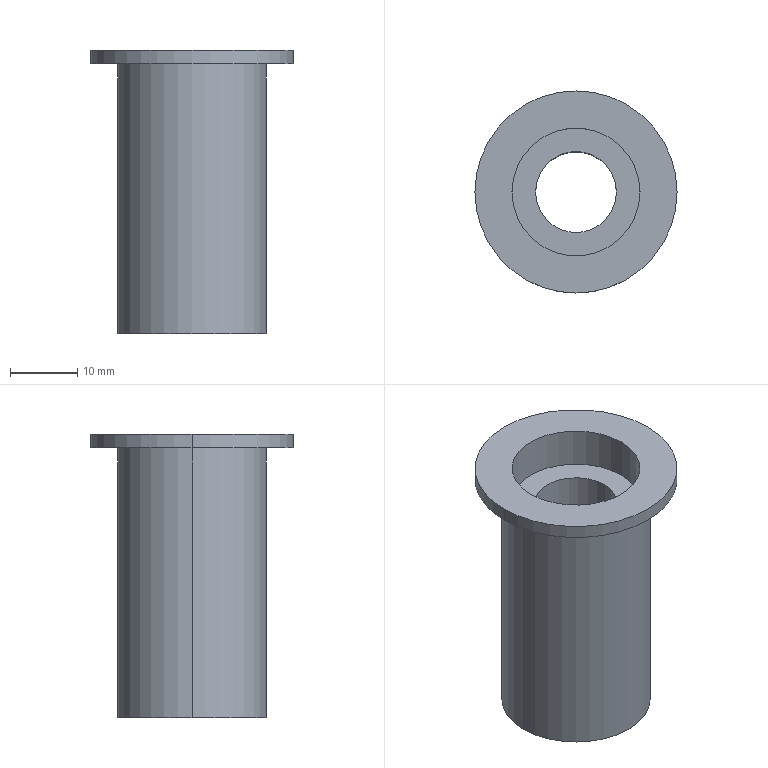Part | STEP file | Tube-changer locating roller SGN-2-21 | 1 solid | 15 faces | box 30 x 30 x 42 mm | volume 9824 mm3 | cylinder 10 | plane 5 | commonest cylinder face diameters 19 x4 12 x2 22 x2 30 x2
STEP:
#1=CARTESIAN_POINT('',(0.,0.,0.));
#2=DIRECTION('',(0.,0.,1.));
#3=DIRECTION('',(1.,0.,0.));
#4=AXIS2_PLACEMENT_3D('',#1,#2,#3);
#5=CARTESIAN_POINT('',(9.5,0.,36.));
#6=VERTEX_POINT('',#5);
#7=CARTESIAN_POINT('',(9.5,0.,42.));
#8=VERTEX_POINT('',#7);
#9=CARTESIAN_POINT('',(9.5,0.,36.));
#10=DIRECTION('',(0.,0.,1.));
#11=VECTOR('',#10,1.);
#12=LINE('',#9,#11);
#13=CARTESIAN_POINT('',(0.,0.,36.));
#14=DIRECTION('',(0.,0.,1.));
#15=DIRECTION('',(1.,0.,0.));
#16=AXIS2_PLACEMENT_3D('',#13,#14,#15);
#17=CYLINDRICAL_SURFACE('',#16,9.5);
#18=CARTESIAN_POINT('',(6.283,0.));
#19=DIRECTION('',(0.,1.));
#20=VECTOR('',#19,1.);
#21=LINE('',#18,#20);
#22=(GEOMETRIC_REPRESENTATION_CONTEXT(2)PARAMETRIC_REPRESENTATION_CONTEXT()REPRESENTATION_CONTEXT('',''));
#23=DEFINITIONAL_REPRESENTATION('',(#21),#22);
#24=PCURVE('',#17,#23);
#25=CARTESIAN_POINT('',(0.,0.,36.));
#26=DIRECTION('',(0.,0.,1.));
#27=DIRECTION('',(1.,0.,0.));
#28=AXIS2_PLACEMENT_3D('',#25,#26,#27);
#29=CYLINDRICAL_SURFACE('',#28,9.5);
#30=CARTESIAN_POINT('',(0.,0.));
#31=DIRECTION('',(0.,1.));
#32=VECTOR('',#31,1.);
#33=LINE('',#30,#32);
#34=(GEOMETRIC_REPRESENTATION_CONTEXT(2)PARAMETRIC_REPRESENTATION_CONTEXT()REPRESENTATION_CONTEXT('',''));
#35=DEFINITIONAL_REPRESENTATION('',(#33),#34);
#36=PCURVE('',#29,#35);
#37=SURFACE_CURVE('',#12,(#24,#36),.PCURVE_S1.);
#38=EDGE_CURVE('',#6,#8,#37,.T.);
#39=ORIENTED_EDGE('',*,*,#38,.T.);
#40=CARTESIAN_POINT('',(-9.5,0.,42.));
#41=VERTEX_POINT('',#40);
#42=CARTESIAN_POINT('',(0.,0.,42.));
#43=DIRECTION('',(0.,0.,1.));
#44=DIRECTION('',(1.,0.,0.));
#45=AXIS2_PLACEMENT_3D('',#42,#43,#44);
#46=CIRCLE('',#45,9.5);
#47=CARTESIAN_POINT('',(0.,6.));
#48=DIRECTION('',(1.,0.));
#49=VECTOR('',#48,1.);
#50=LINE('',#47,#49);
#51=(GEOMETRIC_REPRESENTATION_CONTEXT(2)PARAMETRIC_REPRESENTATION_CONTEXT()REPRESENTATION_CONTEXT('',''));
#52=DEFINITIONAL_REPRESENTATION('',(#50),#51);
#53=PCURVE('',#17,#52);
#54=CARTESIAN_POINT('',(0.,0.,42.));
#55=DIRECTION('',(0.,0.,1.));
#56=DIRECTION('',(1.,0.,0.));
#57=AXIS2_PLACEMENT_3D('',#54,#55,#56);
#58=PLANE('',#57);
#59=CARTESIAN_POINT('',(0.,0.));
#60=DIRECTION('',(1.,0.));
#61=AXIS2_PLACEMENT_2D('',#59,#60);
#62=CIRCLE('',#61,9.5);
#63=(GEOMETRIC_REPRESENTATION_CONTEXT(2)PARAMETRIC_REPRESENTATION_CONTEXT()REPRESENTATION_CONTEXT('',''));
#64=DEFINITIONAL_REPRESENTATION('',(#62),#63);
#65=PCURVE('',#58,#64);
#66=SURFACE_CURVE('',#46,(#53,#65),.PCURVE_S1.);
#67=EDGE_CURVE('',#41,#8,#66,.T.);
#68=ORIENTED_EDGE('',*,*,#67,.F.);
#69=CARTESIAN_POINT('',(-9.5,0.,36.));
#70=VERTEX_POINT('',#69);
#71=CARTESIAN_POINT('',(-9.5,0.,36.));
#72=DIRECTION('',(0.,0.,1.));
#73=VECTOR('',#72,1.);
#74=LINE('',#71,#73);
#75=CARTESIAN_POINT('',(3.142,0.));
#76=DIRECTION('',(0.,1.));
#77=VECTOR('',#76,1.);
#78=LINE('',#75,#77);
#79=(GEOMETRIC_REPRESENTATION_CONTEXT(2)PARAMETRIC_REPRESENTATION_CONTEXT()REPRESENTATION_CONTEXT('',''));
#80=DEFINITIONAL_REPRESENTATION('',(#78),#79);
#81=PCURVE('',#17,#80);
#82=CARTESIAN_POINT('',(3.142,0.));
#83=DIRECTION('',(0.,1.));
#84=VECTOR('',#83,1.);
#85=LINE('',#82,#84);
#86=(GEOMETRIC_REPRESENTATION_CONTEXT(2)PARAMETRIC_REPRESENTATION_CONTEXT()REPRESENTATION_CONTEXT('',''));
#87=DEFINITIONAL_REPRESENTATION('',(#85),#86);
#88=PCURVE('',#29,#87);
#89=SURFACE_CURVE('',#74,(#81,#88),.PCURVE_S1.);
#90=EDGE_CURVE('',#70,#41,#89,.T.);
#91=ORIENTED_EDGE('',*,*,#90,.F.);
#92=CARTESIAN_POINT('',(0.,0.,36.));
#93=DIRECTION('',(0.,0.,1.));
#94=DIRECTION('',(1.,0.,0.));
#95=AXIS2_PLACEMENT_3D('',#92,#93,#94);
#96=CIRCLE('',#95,9.5);
#97=CARTESIAN_POINT('',(0.,0.));
#98=DIRECTION('',(1.,0.));
#99=VECTOR('',#98,1.);
#100=LINE('',#97,#99);
#101=(GEOMETRIC_REPRESENTATION_CONTEXT(2)PARAMETRIC_REPRESENTATION_CONTEXT()REPRESENTATION_CONTEXT('',''));
#102=DEFINITIONAL_REPRESENTATION('',(#100),#101);
#103=PCURVE('',#17,#102);
#104=CARTESIAN_POINT('',(0.,0.,36.));
#105=DIRECTION('',(0.,0.,1.));
#106=DIRECTION('',(1.,0.,0.));
#107=AXIS2_PLACEMENT_3D('',#104,#105,#106);
#108=PLANE('',#107);
#109=CARTESIAN_POINT('',(0.,0.));
#110=DIRECTION('',(1.,0.));
#111=AXIS2_PLACEMENT_2D('',#109,#110);
#112=CIRCLE('',#111,9.5);
#113=(GEOMETRIC_REPRESENTATION_CONTEXT(2)PARAMETRIC_REPRESENTATION_CONTEXT()REPRESENTATION_CONTEXT('',''));
#114=DEFINITIONAL_REPRESENTATION('',(#112),#113);
#115=PCURVE('',#108,#114);
#116=SURFACE_CURVE('',#96,(#103,#115),.PCURVE_S1.);
#117=EDGE_CURVE('',#70,#6,#116,.T.);
#118=ORIENTED_EDGE('',*,*,#117,.T.);
#119=EDGE_LOOP('',(#39,#68,#91,#118));
#120=FACE_BOUND('',#119,.F.);
#121=ADVANCED_FACE('',(#120),#17,.F.);
#122=CARTESIAN_POINT('',(-9.5,0.,6.));
#123=VERTEX_POINT('',#122);
#124=CARTESIAN_POINT('',(-9.5,0.,0.));
#125=VERTEX_POINT('',#124);
#126=CARTESIAN_POINT('',(-9.5,0.,6.));
#127=DIRECTION('',(0.,0.,-1.));
#128=VECTOR('',#127,1.);
#129=LINE('',#126,#128);
#130=CARTESIAN_POINT('',(0.,0.,6.));
#131=DIRECTION('',(0.,0.,-1.));
#132=DIRECTION('',(-1.,0.,0.));
#133=AXIS2_PLACEMENT_3D('',#130,#131,#132);
#134=CYLINDRICAL_SURFACE('',#133,9.5);
#135=CARTESIAN_POINT('',(6.283,0.));
#136=DIRECTION('',(0.,1.));
#137=VECTOR('',#136,1.);
#138=LINE('',#135,#137);
#139=(GEOMETRIC_REPRESENTATION_CONTEXT(2)PARAMETRIC_REPRESENTATION_CONTEXT()REPRESENTATION_CONTEXT('',''));
#140=DEFINITIONAL_REPRESENTATION('',(#138),#139);
#141=PCURVE('',#134,#140);
#142=CARTESIAN_POINT('',(0.,0.,6.));
#143=DIRECTION('',(0.,0.,-1.));
#144=DIRECTION('',(-1.,0.,0.));
#145=AXIS2_PLACEMENT_3D('',#142,#143,#144);
#146=CYLINDRICAL_SURFACE('',#145,9.5);
#147=CARTESIAN_POINT('',(0.,0.));
#148=DIRECTION('',(0.,1.));
#149=VECTOR('',#148,1.);
#150=LINE('',#147,#149);
#151=(GEOMETRIC_REPRESENTATION_CONTEXT(2)PARAMETRIC_REPRESENTATION_CONTEXT()REPRESENTATION_CONTEXT('',''));
#152=DEFINITIONAL_REPRESENTATION('',(#150),#151);
#153=PCURVE('',#146,#152);
#154=SURFACE_CURVE('',#129,(#141,#153),.PCURVE_S1.);
#155=EDGE_CURVE('',#123,#125,#154,.T.);
#156=ORIENTED_EDGE('',*,*,#155,.T.);
#157=CARTESIAN_POINT('',(9.5,0.,0.));
#158=VERTEX_POINT('',#157);
#159=CARTESIAN_POINT('',(0.,0.,0.));
#160=DIRECTION('',(0.,0.,-1.));
#161=DIRECTION('',(-1.,0.,0.));
#162=AXIS2_PLACEMENT_3D('',#159,#160,#161);
#163=CIRCLE('',#162,9.5);
#164=CARTESIAN_POINT('',(0.,6.));
#165=DIRECTION('',(1.,0.));
#166=VECTOR('',#165,1.);
#167=LINE('',#164,#166);
#168=(GEOMETRIC_REPRESENTATION_CONTEXT(2)PARAMETRIC_REPRESENTATION_CONTEXT()REPRESENTATION_CONTEXT('',''));
#169=DEFINITIONAL_REPRESENTATION('',(#167),#168);
#170=PCURVE('',#134,#169);
#171=CARTESIAN_POINT('',(0.,0.,0.));
#172=DIRECTION('',(0.,0.,1.));
#173=DIRECTION('',(1.,0.,0.));
#174=AXIS2_PLACEMENT_3D('',#171,#172,#173);
#175=PLANE('',#174);
#176=CARTESIAN_POINT('',(-9.5,0.));
#177=CARTESIAN_POINT('',(-9.5,16.454));
#178=CARTESIAN_POINT('',(4.75,8.227));
#179=CARTESIAN_POINT('',(19.,0.));
#180=CARTESIAN_POINT('',(4.75,-8.227));
#181=CARTESIAN_POINT('',(-9.5,-16.454));
#182=CARTESIAN_POINT('',(-9.5,0.));
#183=(BOUNDED_CURVE()B_SPLINE_CURVE(2,(#176,#177,#178,#179,#180,#181,#182),.UNSPECIFIED.,.T.,.F.)B_SPLINE_CURVE_WITH_KNOTS((1,2,2,2,2,1),(-2.094,0.,2.094,4.189,6.283,8.378),.UNSPECIFIED.)CURVE()GEOMETRIC_REPRESENTATION_ITEM()RATIONAL_B_SPLINE_CURVE((1.,0.5,1.,0.5,1.,0.5,1.))REPRESENTATION_ITEM(''));
#184=(GEOMETRIC_REPRESENTATION_CONTEXT(2)PARAMETRIC_REPRESENTATION_CONTEXT()REPRESENTATION_CONTEXT('',''));
#185=DEFINITIONAL_REPRESENTATION('',(#183),#184);
#186=PCURVE('',#175,#185);
#187=SURFACE_CURVE('',#163,(#170,#186),.PCURVE_S1.);
#188=EDGE_CURVE('',#158,#125,#187,.T.);
#189=ORIENTED_EDGE('',*,*,#188,.F.);
#190=CARTESIAN_POINT('',(9.5,0.,6.));
#191=VERTEX_POINT('',#190);
#192=CARTESIAN_POINT('',(9.5,0.,6.));
#193=DIRECTION('',(0.,0.,-1.));
#194=VECTOR('',#193,1.);
#195=LINE('',#192,#194);
#196=CARTESIAN_POINT('',(3.142,0.));
#197=DIRECTION('',(0.,1.));
#198=VECTOR('',#197,1.);
#199=LINE('',#196,#198);
#200=(GEOMETRIC_REPRESENTATION_CONTEXT(2)PARAMETRIC_REPRESENTATION_CONTEXT()REPRESENTATION_CONTEXT('',''));
#201=DEFINITIONAL_REPRESENTATION('',(#199),#200);
#202=PCURVE('',#134,#201);
#203=CARTESIAN_POINT('',(3.142,0.));
#204=DIRECTION('',(0.,1.));
#205=VECTOR('',#204,1.);
#206=LINE('',#203,#205);
#207=(GEOMETRIC_REPRESENTATION_CONTEXT(2)PARAMETRIC_REPRESENTATION_CONTEXT()REPRESENTATION_CONTEXT('',''));
#208=DEFINITIONAL_REPRESENTATION('',(#206),#207);
#209=PCURVE('',#146,#208);
#210=SURFACE_CURVE('',#195,(#202,#209),.PCURVE_S1.);
#211=EDGE_CURVE('',#191,#158,#210,.T.);
#212=ORIENTED_EDGE('',*,*,#211,.F.);
#213=CARTESIAN_POINT('',(0.,0.,6.));
#214=DIRECTION('',(0.,0.,-1.));
#215=DIRECTION('',(-1.,0.,0.));
#216=AXIS2_PLACEMENT_3D('',#213,#214,#215);
#217=CIRCLE('',#216,9.5);
#218=CARTESIAN_POINT('',(0.,0.));
#219=DIRECTION('',(1.,0.));
#220=VECTOR('',#219,1.);
#221=LINE('',#218,#220);
#222=(GEOMETRIC_REPRESENTATION_CONTEXT(2)PARAMETRIC_REPRESENTATION_CONTEXT()REPRESENTATION_CONTEXT('',''));
#223=DEFINITIONAL_REPRESENTATION('',(#221),#222);
#224=PCURVE('',#134,#223);
#225=CARTESIAN_POINT('',(0.,0.,6.));
#226=DIRECTION('',(0.,0.,-1.));
#227=DIRECTION('',(-1.,0.,0.));
#228=AXIS2_PLACEMENT_3D('',#225,#226,#227);
#229=PLANE('',#228);
#230=CARTESIAN_POINT('',(0.,0.));
#231=DIRECTION('',(1.,0.));
#232=AXIS2_PLACEMENT_2D('',#230,#231);
#233=CIRCLE('',#232,9.5);
#234=(GEOMETRIC_REPRESENTATION_CONTEXT(2)PARAMETRIC_REPRESENTATION_CONTEXT()REPRESENTATION_CONTEXT('',''));
#235=DEFINITIONAL_REPRESENTATION('',(#233),#234);
#236=PCURVE('',#229,#235);
#237=SURFACE_CURVE('',#217,(#224,#236),.PCURVE_S1.);
#238=EDGE_CURVE('',#191,#123,#237,.T.);
#239=ORIENTED_EDGE('',*,*,#238,.T.);
#240=EDGE_LOOP('',(#156,#189,#212,#239));
#241=FACE_BOUND('',#240,.F.);
#242=ADVANCED_FACE('',(#241),#134,.F.);
#243=CARTESIAN_POINT('',(15.,0.,42.));
#244=VERTEX_POINT('',#243);
#245=CARTESIAN_POINT('',(-15.,0.,42.));
#246=VERTEX_POINT('',#245);
#247=CARTESIAN_POINT('',(0.,0.,42.));
#248=DIRECTION('',(0.,0.,1.));
#249=DIRECTION('',(1.,0.,0.));
#250=AXIS2_PLACEMENT_3D('',#247,#248,#249);
#251=CIRCLE('',#250,15.);
#252=CARTESIAN_POINT('',(0.,0.,42.));
#253=DIRECTION('',(0.,0.,-1.));
#254=DIRECTION('',(-1.,0.,0.));
#255=AXIS2_PLACEMENT_3D('',#252,#253,#254);
#256=CYLINDRICAL_SURFACE('',#255,15.);
#257=CARTESIAN_POINT('',(3.142,0.));
#258=DIRECTION('',(-1.,0.));
#259=VECTOR('',#258,1.);
#260=LINE('',#257,#259);
#261=(GEOMETRIC_REPRESENTATION_CONTEXT(2)PARAMETRIC_REPRESENTATION_CONTEXT()REPRESENTATION_CONTEXT('',''));
#262=DEFINITIONAL_REPRESENTATION('',(#260),#261);
#263=PCURVE('',#256,#262);
#264=CARTESIAN_POINT('',(0.,0.));
#265=DIRECTION('',(1.,0.));
#266=AXIS2_PLACEMENT_2D('',#264,#265);
#267=CIRCLE('',#266,15.);
#268=(GEOMETRIC_REPRESENTATION_CONTEXT(2)PARAMETRIC_REPRESENTATION_CONTEXT()REPRESENTATION_CONTEXT('',''));
#269=DEFINITIONAL_REPRESENTATION('',(#267),#268);
#270=PCURVE('',#58,#269);
#271=SURFACE_CURVE('',#251,(#263,#270),.PCURVE_S1.);
#272=EDGE_CURVE('',#244,#246,#271,.T.);
#273=ORIENTED_EDGE('',*,*,#272,.F.);
#274=CARTESIAN_POINT('',(15.,0.,40.));
#275=VERTEX_POINT('',#274);
#276=CARTESIAN_POINT('',(15.,0.,42.));
#277=DIRECTION('',(0.,0.,-1.));
#278=VECTOR('',#277,1.);
#279=LINE('',#276,#278);
#280=CARTESIAN_POINT('',(3.142,0.));
#281=DIRECTION('',(0.,1.));
#282=VECTOR('',#281,1.);
#283=LINE('',#280,#282);
#284=(GEOMETRIC_REPRESENTATION_CONTEXT(2)PARAMETRIC_REPRESENTATION_CONTEXT()REPRESENTATION_CONTEXT('',''));
#285=DEFINITIONAL_REPRESENTATION('',(#283),#284);
#286=PCURVE('',#256,#285);
#287=CARTESIAN_POINT('',(0.,0.,42.));
#288=DIRECTION('',(0.,0.,-1.));
#289=DIRECTION('',(-1.,0.,0.));
#290=AXIS2_PLACEMENT_3D('',#287,#288,#289);
#291=CYLINDRICAL_SURFACE('',#290,15.);
#292=CARTESIAN_POINT('',(3.142,0.));
#293=DIRECTION('',(0.,1.));
#294=VECTOR('',#293,1.);
#295=LINE('',#292,#294);
#296=(GEOMETRIC_REPRESENTATION_CONTEXT(2)PARAMETRIC_REPRESENTATION_CONTEXT()REPRESENTATION_CONTEXT('',''));
#297=DEFINITIONAL_REPRESENTATION('',(#295),#296);
#298=PCURVE('',#291,#297);
#299=SURFACE_CURVE('',#279,(#286,#298),.PCURVE_S1.);
#300=EDGE_CURVE('',#244,#275,#299,.T.);
#301=ORIENTED_EDGE('',*,*,#300,.T.);
#302=CARTESIAN_POINT('',(-15.,0.,40.));
#303=VERTEX_POINT('',#302);
#304=CARTESIAN_POINT('',(0.,0.,40.));
#305=DIRECTION('',(0.,0.,1.));
#306=DIRECTION('',(1.,0.,0.));
#307=AXIS2_PLACEMENT_3D('',#304,#305,#306);
#308=CIRCLE('',#307,15.);
#309=CARTESIAN_POINT('',(3.142,2.));
#310=DIRECTION('',(-1.,0.));
#311=VECTOR('',#310,1.);
#312=LINE('',#309,#311);
#313=(GEOMETRIC_REPRESENTATION_CONTEXT(2)PARAMETRIC_REPRESENTATION_CONTEXT()REPRESENTATION_CONTEXT('',''));
#314=DEFINITIONAL_REPRESENTATION('',(#312),#313);
#315=PCURVE('',#256,#314);
#316=CARTESIAN_POINT('',(0.,0.,40.));
#317=DIRECTION('',(0.,0.,1.));
#318=DIRECTION('',(1.,0.,0.));
#319=AXIS2_PLACEMENT_3D('',#316,#317,#318);
#320=PLANE('',#319);
#321=CARTESIAN_POINT('',(0.,0.));
#322=DIRECTION('',(1.,0.));
#323=AXIS2_PLACEMENT_2D('',#321,#322);
#324=CIRCLE('',#323,15.);
#325=(GEOMETRIC_REPRESENTATION_CONTEXT(2)PARAMETRIC_REPRESENTATION_CONTEXT()REPRESENTATION_CONTEXT('',''));
#326=DEFINITIONAL_REPRESENTATION('',(#324),#325);
#327=PCURVE('',#320,#326);
#328=SURFACE_CURVE('',#308,(#315,#327),.PCURVE_S1.);
#329=EDGE_CURVE('',#275,#303,#328,.T.);
#330=ORIENTED_EDGE('',*,*,#329,.T.);
#331=CARTESIAN_POINT('',(-15.,0.,42.));
#332=DIRECTION('',(0.,0.,-1.));
#333=VECTOR('',#332,1.);
#334=LINE('',#331,#333);
#335=CARTESIAN_POINT('',(0.,0.));
#336=DIRECTION('',(0.,1.));
#337=VECTOR('',#336,1.);
#338=LINE('',#335,#337);
#339=(GEOMETRIC_REPRESENTATION_CONTEXT(2)PARAMETRIC_REPRESENTATION_CONTEXT()REPRESENTATION_CONTEXT('',''));
#340=DEFINITIONAL_REPRESENTATION('',(#338),#339);
#341=PCURVE('',#256,#340);
#342=CARTESIAN_POINT('',(6.283,0.));
#343=DIRECTION('',(0.,1.));
#344=VECTOR('',#343,1.);
#345=LINE('',#342,#344);
#346=(GEOMETRIC_REPRESENTATION_CONTEXT(2)PARAMETRIC_REPRESENTATION_CONTEXT()REPRESENTATION_CONTEXT('',''));
#347=DEFINITIONAL_REPRESENTATION('',(#345),#346);
#348=PCURVE('',#291,#347);
#349=SURFACE_CURVE('',#334,(#341,#348),.PCURVE_S1.);
#350=EDGE_CURVE('',#246,#303,#349,.T.);
#351=ORIENTED_EDGE('',*,*,#350,.F.);
#352=EDGE_LOOP('',(#273,#301,#330,#351));
#353=FACE_BOUND('',#352,.T.);
#354=ADVANCED_FACE('',(#353),#256,.T.);
#355=CARTESIAN_POINT('',(11.,0.,40.));
#356=VERTEX_POINT('',#355);
#357=CARTESIAN_POINT('',(-11.,0.,40.));
#358=VERTEX_POINT('',#357);
#359=CARTESIAN_POINT('',(0.,0.,40.));
#360=DIRECTION('',(0.,0.,1.));
#361=DIRECTION('',(1.,0.,0.));
#362=AXIS2_PLACEMENT_3D('',#359,#360,#361);
#363=CIRCLE('',#362,11.);
#364=CARTESIAN_POINT('',(0.,0.,40.));
#365=DIRECTION('',(0.,0.,-1.));
#366=DIRECTION('',(-1.,0.,0.));
#367=AXIS2_PLACEMENT_3D('',#364,#365,#366);
#368=CYLINDRICAL_SURFACE('',#367,11.);
#369=CARTESIAN_POINT('',(3.142,0.));
#370=DIRECTION('',(-1.,0.));
#371=VECTOR('',#370,1.);
#372=LINE('',#369,#371);
#373=(GEOMETRIC_REPRESENTATION_CONTEXT(2)PARAMETRIC_REPRESENTATION_CONTEXT()REPRESENTATION_CONTEXT('',''));
#374=DEFINITIONAL_REPRESENTATION('',(#372),#373);
#375=PCURVE('',#368,#374);
#376=CARTESIAN_POINT('',(0.,0.));
#377=DIRECTION('',(1.,0.));
#378=AXIS2_PLACEMENT_2D('',#376,#377);
#379=CIRCLE('',#378,11.);
#380=(GEOMETRIC_REPRESENTATION_CONTEXT(2)PARAMETRIC_REPRESENTATION_CONTEXT()REPRESENTATION_CONTEXT('',''));
#381=DEFINITIONAL_REPRESENTATION('',(#379),#380);
#382=PCURVE('',#320,#381);
#383=SURFACE_CURVE('',#363,(#375,#382),.PCURVE_S1.);
#384=EDGE_CURVE('',#356,#358,#383,.T.);
#385=ORIENTED_EDGE('',*,*,#384,.F.);
#386=CARTESIAN_POINT('',(11.,0.,0.));
#387=VERTEX_POINT('',#386);
#388=CARTESIAN_POINT('',(11.,0.,40.));
#389=DIRECTION('',(0.,0.,-1.));
#390=VECTOR('',#389,1.);
#391=LINE('',#388,#390);
#392=CARTESIAN_POINT('',(3.142,0.));
#393=DIRECTION('',(0.,1.));
#394=VECTOR('',#393,1.);
#395=LINE('',#392,#394);
#396=(GEOMETRIC_REPRESENTATION_CONTEXT(2)PARAMETRIC_REPRESENTATION_CONTEXT()REPRESENTATION_CONTEXT('',''));
#397=DEFINITIONAL_REPRESENTATION('',(#395),#396);
#398=PCURVE('',#368,#397);
#399=CARTESIAN_POINT('',(0.,0.,40.));
#400=DIRECTION('',(0.,0.,-1.));
#401=DIRECTION('',(-1.,0.,0.));
#402=AXIS2_PLACEMENT_3D('',#399,#400,#401);
#403=CYLINDRICAL_SURFACE('',#402,11.);
#404=CARTESIAN_POINT('',(3.142,0.));
#405=DIRECTION('',(0.,1.));
#406=VECTOR('',#405,1.);
#407=LINE('',#404,#406);
#408=(GEOMETRIC_REPRESENTATION_CONTEXT(2)PARAMETRIC_REPRESENTATION_CONTEXT()REPRESENTATION_CONTEXT('',''));
#409=DEFINITIONAL_REPRESENTATION('',(#407),#408);
#410=PCURVE('',#403,#409);
#411=SURFACE_CURVE('',#391,(#398,#410),.PCURVE_S1.);
#412=EDGE_CURVE('',#356,#387,#411,.T.);
#413=ORIENTED_EDGE('',*,*,#412,.T.);
#414=CARTESIAN_POINT('',(-11.,0.,0.));
#415=VERTEX_POINT('',#414);
#416=CARTESIAN_POINT('',(0.,0.,0.));
#417=DIRECTION('',(0.,0.,1.));
#418=DIRECTION('',(1.,0.,0.));
#419=AXIS2_PLACEMENT_3D('',#416,#417,#418);
#420=CIRCLE('',#419,11.);
#421=CARTESIAN_POINT('',(3.142,40.));
#422=DIRECTION('',(-1.,0.));
#423=VECTOR('',#422,1.);
#424=LINE('',#421,#423);
#425=(GEOMETRIC_REPRESENTATION_CONTEXT(2)PARAMETRIC_REPRESENTATION_CONTEXT()REPRESENTATION_CONTEXT('',''));
#426=DEFINITIONAL_REPRESENTATION('',(#424),#425);
#427=PCURVE('',#368,#426);
#428=CARTESIAN_POINT('',(0.,0.));
#429=DIRECTION('',(1.,0.));
#430=AXIS2_PLACEMENT_2D('',#428,#429);
#431=CIRCLE('',#430,11.);
#432=(GEOMETRIC_REPRESENTATION_CONTEXT(2)PARAMETRIC_REPRESENTATION_CONTEXT()REPRESENTATION_CONTEXT('',''));
#433=DEFINITIONAL_REPRESENTATION('',(#431),#432);
#434=PCURVE('',#175,#433);
#435=SURFACE_CURVE('',#420,(#427,#434),.PCURVE_S1.);
#436=EDGE_CURVE('',#387,#415,#435,.T.);
#437=ORIENTED_EDGE('',*,*,#436,.T.);
#438=CARTESIAN_POINT('',(-11.,0.,40.));
#439=DIRECTION('',(0.,0.,-1.));
#440=VECTOR('',#439,1.);
#441=LINE('',#438,#440);
#442=CARTESIAN_POINT('',(0.,0.));
#443=DIRECTION('',(0.,1.));
#444=VECTOR('',#443,1.);
#445=LINE('',#442,#444);
#446=(GEOMETRIC_REPRESENTATION_CONTEXT(2)PARAMETRIC_REPRESENTATION_CONTEXT()REPRESENTATION_CONTEXT('',''));
#447=DEFINITIONAL_REPRESENTATION('',(#445),#446);
#448=PCURVE('',#368,#447);
#449=CARTESIAN_POINT('',(6.283,0.));
#450=DIRECTION('',(0.,1.));
#451=VECTOR('',#450,1.);
#452=LINE('',#449,#451);
#453=(GEOMETRIC_REPRESENTATION_CONTEXT(2)PARAMETRIC_REPRESENTATION_CONTEXT()REPRESENTATION_CONTEXT('',''));
#454=DEFINITIONAL_REPRESENTATION('',(#452),#453);
#455=PCURVE('',#403,#454);
#456=SURFACE_CURVE('',#441,(#448,#455),.PCURVE_S1.);
#457=EDGE_CURVE('',#358,#415,#456,.T.);
#458=ORIENTED_EDGE('',*,*,#457,.F.);
#459=EDGE_LOOP('',(#385,#413,#437,#458));
#460=FACE_BOUND('',#459,.T.);
#461=ADVANCED_FACE('',(#460),#368,.T.);
#462=CARTESIAN_POINT('',(-6.,0.,36.));
#463=VERTEX_POINT('',#462);
#464=CARTESIAN_POINT('',(-6.,0.,6.));
#465=VERTEX_POINT('',#464);
#466=CARTESIAN_POINT('',(-6.,0.,40.));
#467=DIRECTION('',(0.,0.,-1.));
#468=VECTOR('',#467,1.);
#469=LINE('',#466,#468);
#470=CARTESIAN_POINT('',(0.,0.,40.));
#471=DIRECTION('',(0.,0.,-1.));
#472=DIRECTION('',(-1.,0.,0.));
#473=AXIS2_PLACEMENT_3D('',#470,#471,#472);
#474=CYLINDRICAL_SURFACE('',#473,6.);
#475=CARTESIAN_POINT('',(6.283,0.));
#476=DIRECTION('',(0.,1.));
#477=VECTOR('',#476,1.);
#478=LINE('',#475,#477);
#479=(GEOMETRIC_REPRESENTATION_CONTEXT(2)PARAMETRIC_REPRESENTATION_CONTEXT()REPRESENTATION_CONTEXT('',''));
#480=DEFINITIONAL_REPRESENTATION('',(#478),#479);
#481=PCURVE('',#474,#480);
#482=CARTESIAN_POINT('',(0.,0.,40.));
#483=DIRECTION('',(0.,0.,-1.));
#484=DIRECTION('',(-1.,0.,0.));
#485=AXIS2_PLACEMENT_3D('',#482,#483,#484);
#486=CYLINDRICAL_SURFACE('',#485,6.);
#487=CARTESIAN_POINT('',(0.,0.));
#488=DIRECTION('',(0.,1.));
#489=VECTOR('',#488,1.);
#490=LINE('',#487,#489);
#491=(GEOMETRIC_REPRESENTATION_CONTEXT(2)PARAMETRIC_REPRESENTATION_CONTEXT()REPRESENTATION_CONTEXT('',''));
#492=DEFINITIONAL_REPRESENTATION('',(#490),#491);
#493=PCURVE('',#486,#492);
#494=SURFACE_CURVE('',#469,(#481,#493),.PCURVE_S1.);
#495=EDGE_CURVE('',#463,#465,#494,.T.);
#496=ORIENTED_EDGE('',*,*,#495,.T.);
#497=CARTESIAN_POINT('',(6.,0.,6.));
#498=VERTEX_POINT('',#497);
#499=CARTESIAN_POINT('',(0.,0.,6.));
#500=DIRECTION('',(0.,0.,-1.));
#501=DIRECTION('',(-1.,0.,0.));
#502=AXIS2_PLACEMENT_3D('',#499,#500,#501);
#503=CIRCLE('',#502,6.);
#504=CARTESIAN_POINT('',(0.,34.));
#505=DIRECTION('',(1.,0.));
#506=VECTOR('',#505,1.);
#507=LINE('',#504,#506);
#508=(GEOMETRIC_REPRESENTATION_CONTEXT(2)PARAMETRIC_REPRESENTATION_CONTEXT()REPRESENTATION_CONTEXT('',''));
#509=DEFINITIONAL_REPRESENTATION('',(#507),#508);
#510=PCURVE('',#474,#509);
#511=CARTESIAN_POINT('',(0.,0.));
#512=DIRECTION('',(1.,0.));
#513=AXIS2_PLACEMENT_2D('',#511,#512);
#514=CIRCLE('',#513,6.);
#515=(GEOMETRIC_REPRESENTATION_CONTEXT(2)PARAMETRIC_REPRESENTATION_CONTEXT()REPRESENTATION_CONTEXT('',''));
#516=DEFINITIONAL_REPRESENTATION('',(#514),#515);
#517=PCURVE('',#229,#516);
#518=SURFACE_CURVE('',#503,(#510,#517),.PCURVE_S1.);
#519=EDGE_CURVE('',#498,#465,#518,.T.);
#520=ORIENTED_EDGE('',*,*,#519,.F.);
#521=CARTESIAN_POINT('',(6.,0.,36.));
#522=VERTEX_POINT('',#521);
#523=CARTESIAN_POINT('',(6.,0.,40.));
#524=DIRECTION('',(0.,0.,-1.));
#525=VECTOR('',#524,1.);
#526=LINE('',#523,#525);
#527=CARTESIAN_POINT('',(3.142,0.));
#528=DIRECTION('',(0.,1.));
#529=VECTOR('',#528,1.);
#530=LINE('',#527,#529);
#531=(GEOMETRIC_REPRESENTATION_CONTEXT(2)PARAMETRIC_REPRESENTATION_CONTEXT()REPRESENTATION_CONTEXT('',''));
#532=DEFINITIONAL_REPRESENTATION('',(#530),#531);
#533=PCURVE('',#474,#532);
#534=CARTESIAN_POINT('',(3.142,0.));
#535=DIRECTION('',(0.,1.));
#536=VECTOR('',#535,1.);
#537=LINE('',#534,#536);
#538=(GEOMETRIC_REPRESENTATION_CONTEXT(2)PARAMETRIC_REPRESENTATION_CONTEXT()REPRESENTATION_CONTEXT('',''));
#539=DEFINITIONAL_REPRESENTATION('',(#537),#538);
#540=PCURVE('',#486,#539);
#541=SURFACE_CURVE('',#526,(#533,#540),.PCURVE_S1.);
#542=EDGE_CURVE('',#522,#498,#541,.T.);
#543=ORIENTED_EDGE('',*,*,#542,.F.);
#544=CARTESIAN_POINT('',(0.,0.,36.));
#545=DIRECTION('',(0.,0.,1.));
#546=DIRECTION('',(1.,0.,0.));
#547=AXIS2_PLACEMENT_3D('',#544,#545,#546);
#548=CIRCLE('',#547,6.);
#549=CARTESIAN_POINT('',(9.425,4.));
#550=DIRECTION('',(-1.,0.));
#551=VECTOR('',#550,1.);
#552=LINE('',#549,#551);
#553=(GEOMETRIC_REPRESENTATION_CONTEXT(2)PARAMETRIC_REPRESENTATION_CONTEXT()REPRESENTATION_CONTEXT('',''));
#554=DEFINITIONAL_REPRESENTATION('',(#552),#553);
#555=PCURVE('',#474,#554);
#556=CARTESIAN_POINT('',(0.,0.));
#557=DIRECTION('',(1.,0.));
#558=AXIS2_PLACEMENT_2D('',#556,#557);
#559=CIRCLE('',#558,6.);
#560=(GEOMETRIC_REPRESENTATION_CONTEXT(2)PARAMETRIC_REPRESENTATION_CONTEXT()REPRESENTATION_CONTEXT('',''));
#561=DEFINITIONAL_REPRESENTATION('',(#559),#560);
#562=PCURVE('',#108,#561);
#563=SURFACE_CURVE('',#548,(#555,#562),.PCURVE_S1.);
#564=EDGE_CURVE('',#463,#522,#563,.T.);
#565=ORIENTED_EDGE('',*,*,#564,.F.);
#566=EDGE_LOOP('',(#496,#520,#543,#565));
#567=FACE_BOUND('',#566,.F.);
#568=ADVANCED_FACE('',(#567),#474,.F.);
#569=CARTESIAN_POINT('',(0.,0.,6.));
#570=DIRECTION('',(0.,0.,-1.));
#571=DIRECTION('',(-1.,0.,0.));
#572=AXIS2_PLACEMENT_3D('',#569,#570,#571);
#573=CIRCLE('',#572,6.);
#574=CARTESIAN_POINT('',(0.,34.));
#575=DIRECTION('',(1.,0.));
#576=VECTOR('',#575,1.);
#577=LINE('',#574,#576);
#578=(GEOMETRIC_REPRESENTATION_CONTEXT(2)PARAMETRIC_REPRESENTATION_CONTEXT()REPRESENTATION_CONTEXT('',''));
#579=DEFINITIONAL_REPRESENTATION('',(#577),#578);
#580=PCURVE('',#486,#579);
#581=CARTESIAN_POINT('',(0.,0.));
#582=DIRECTION('',(1.,0.));
#583=AXIS2_PLACEMENT_2D('',#581,#582);
#584=CIRCLE('',#583,6.);
#585=(GEOMETRIC_REPRESENTATION_CONTEXT(2)PARAMETRIC_REPRESENTATION_CONTEXT()REPRESENTATION_CONTEXT('',''));
#586=DEFINITIONAL_REPRESENTATION('',(#584),#585);
#587=PCURVE('',#229,#586);
#588=SURFACE_CURVE('',#573,(#580,#587),.PCURVE_S1.);
#589=EDGE_CURVE('',#465,#498,#588,.T.);
#590=ORIENTED_EDGE('',*,*,#589,.F.);
#591=ORIENTED_EDGE('',*,*,#495,.F.);
#592=CARTESIAN_POINT('',(0.,0.,36.));
#593=DIRECTION('',(0.,0.,1.));
#594=DIRECTION('',(1.,0.,0.));
#595=AXIS2_PLACEMENT_3D('',#592,#593,#594);
#596=CIRCLE('',#595,6.);
#597=CARTESIAN_POINT('',(3.142,4.));
#598=DIRECTION('',(-1.,0.));
#599=VECTOR('',#598,1.);
#600=LINE('',#597,#599);
#601=(GEOMETRIC_REPRESENTATION_CONTEXT(2)PARAMETRIC_REPRESENTATION_CONTEXT()REPRESENTATION_CONTEXT('',''));
#602=DEFINITIONAL_REPRESENTATION('',(#600),#601);
#603=PCURVE('',#486,#602);
#604=CARTESIAN_POINT('',(0.,0.));
#605=DIRECTION('',(1.,0.));
#606=AXIS2_PLACEMENT_2D('',#604,#605);
#607=CIRCLE('',#606,6.);
#608=(GEOMETRIC_REPRESENTATION_CONTEXT(2)PARAMETRIC_REPRESENTATION_CONTEXT()REPRESENTATION_CONTEXT('',''));
#609=DEFINITIONAL_REPRESENTATION('',(#607),#608);
#610=PCURVE('',#108,#609);
#611=SURFACE_CURVE('',#596,(#603,#610),.PCURVE_S1.);
#612=EDGE_CURVE('',#522,#463,#611,.T.);
#613=ORIENTED_EDGE('',*,*,#612,.F.);
#614=ORIENTED_EDGE('',*,*,#542,.T.);
#615=EDGE_LOOP('',(#590,#591,#613,#614));
#616=FACE_BOUND('',#615,.F.);
#617=ADVANCED_FACE('',(#616),#486,.F.);
#618=CARTESIAN_POINT('',(0.,0.,0.));
#619=DIRECTION('',(0.,0.,-1.));
#620=DIRECTION('',(-1.,0.,0.));
#621=AXIS2_PLACEMENT_3D('',#618,#619,#620);
#622=CIRCLE('',#621,9.5);
#623=CARTESIAN_POINT('',(-9.5,0.));
#624=CARTESIAN_POINT('',(-9.5,16.454));
#625=CARTESIAN_POINT('',(4.75,8.227));
#626=CARTESIAN_POINT('',(19.,0.));
#627=CARTESIAN_POINT('',(4.75,-8.227));
#628=CARTESIAN_POINT('',(-9.5,-16.454));
#629=CARTESIAN_POINT('',(-9.5,0.));
#630=(BOUNDED_CURVE()B_SPLINE_CURVE(2,(#623,#624,#625,#626,#627,#628,#629),.UNSPECIFIED.,.T.,.F.)B_SPLINE_CURVE_WITH_KNOTS((1,2,2,2,2,1),(-2.094,0.,2.094,4.189,6.283,8.378),.UNSPECIFIED.)CURVE()GEOMETRIC_REPRESENTATION_ITEM()RATIONAL_B_SPLINE_CURVE((1.,0.5,1.,0.5,1.,0.5,1.))REPRESENTATION_ITEM(''));
#631=(GEOMETRIC_REPRESENTATION_CONTEXT(2)PARAMETRIC_REPRESENTATION_CONTEXT()REPRESENTATION_CONTEXT('',''));
#632=DEFINITIONAL_REPRESENTATION('',(#630),#631);
#633=PCURVE('',#175,#632);
#634=CARTESIAN_POINT('',(0.,6.));
#635=DIRECTION('',(1.,0.));
#636=VECTOR('',#635,1.);
#637=LINE('',#634,#636);
#638=(GEOMETRIC_REPRESENTATION_CONTEXT(2)PARAMETRIC_REPRESENTATION_CONTEXT()REPRESENTATION_CONTEXT('',''));
#639=DEFINITIONAL_REPRESENTATION('',(#637),#638);
#640=PCURVE('',#146,#639);
#641=SURFACE_CURVE('',#622,(#633,#640),.PCURVE_S1.);
#642=EDGE_CURVE('',#125,#158,#641,.T.);
#643=ORIENTED_EDGE('',*,*,#642,.F.);
#644=ORIENTED_EDGE('',*,*,#188,.F.);
#645=EDGE_LOOP('',(#643,#644));
#646=FACE_BOUND('',#645,.T.);
#647=CARTESIAN_POINT('',(0.,0.,0.));
#648=DIRECTION('',(0.,0.,1.));
#649=DIRECTION('',(1.,0.,0.));
#650=AXIS2_PLACEMENT_3D('',#647,#648,#649);
#651=CIRCLE('',#650,11.);
#652=CARTESIAN_POINT('',(0.,0.));
#653=DIRECTION('',(1.,0.));
#654=AXIS2_PLACEMENT_2D('',#652,#653);
#655=CIRCLE('',#654,11.);
#656=(GEOMETRIC_REPRESENTATION_CONTEXT(2)PARAMETRIC_REPRESENTATION_CONTEXT()REPRESENTATION_CONTEXT('',''));
#657=DEFINITIONAL_REPRESENTATION('',(#655),#656);
#658=PCURVE('',#175,#657);
#659=CARTESIAN_POINT('',(9.425,40.));
#660=DIRECTION('',(-1.,0.));
#661=VECTOR('',#660,1.);
#662=LINE('',#659,#661);
#663=(GEOMETRIC_REPRESENTATION_CONTEXT(2)PARAMETRIC_REPRESENTATION_CONTEXT()REPRESENTATION_CONTEXT('',''));
#664=DEFINITIONAL_REPRESENTATION('',(#662),#663);
#665=PCURVE('',#403,#664);
#666=SURFACE_CURVE('',#651,(#658,#665),.PCURVE_S1.);
#667=EDGE_CURVE('',#415,#387,#666,.T.);
#668=ORIENTED_EDGE('',*,*,#667,.F.);
#669=ORIENTED_EDGE('',*,*,#436,.F.);
#670=EDGE_LOOP('',(#668,#669));
#671=FACE_BOUND('',#670,.T.);
#672=ADVANCED_FACE('',(#646,#671),#175,.F.);
#673=ORIENTED_EDGE('',*,*,#412,.F.);
#674=CARTESIAN_POINT('',(0.,0.,40.));
#675=DIRECTION('',(0.,0.,1.));
#676=DIRECTION('',(1.,0.,0.));
#677=AXIS2_PLACEMENT_3D('',#674,#675,#676);
#678=CIRCLE('',#677,11.);
#679=CARTESIAN_POINT('',(9.425,0.));
#680=DIRECTION('',(-1.,0.));
#681=VECTOR('',#680,1.);
#682=LINE('',#679,#681);
#683=(GEOMETRIC_REPRESENTATION_CONTEXT(2)PARAMETRIC_REPRESENTATION_CONTEXT()REPRESENTATION_CONTEXT('',''));
#684=DEFINITIONAL_REPRESENTATION('',(#682),#683);
#685=PCURVE('',#403,#684);
#686=CARTESIAN_POINT('',(0.,0.));
#687=DIRECTION('',(1.,0.));
#688=AXIS2_PLACEMENT_2D('',#686,#687);
#689=CIRCLE('',#688,11.);
#690=(GEOMETRIC_REPRESENTATION_CONTEXT(2)PARAMETRIC_REPRESENTATION_CONTEXT()REPRESENTATION_CONTEXT('',''));
#691=DEFINITIONAL_REPRESENTATION('',(#689),#690);
#692=PCURVE('',#320,#691);
#693=SURFACE_CURVE('',#678,(#685,#692),.PCURVE_S1.);
#694=EDGE_CURVE('',#358,#356,#693,.T.);
#695=ORIENTED_EDGE('',*,*,#694,.F.);
#696=ORIENTED_EDGE('',*,*,#457,.T.);
#697=ORIENTED_EDGE('',*,*,#667,.T.);
#698=EDGE_LOOP('',(#673,#695,#696,#697));
#699=FACE_BOUND('',#698,.T.);
#700=ADVANCED_FACE('',(#699),#403,.T.);
#701=CARTESIAN_POINT('',(0.,0.,42.));
#702=DIRECTION('',(0.,0.,1.));
#703=DIRECTION('',(1.,0.,0.));
#704=AXIS2_PLACEMENT_3D('',#701,#702,#703);
#705=CIRCLE('',#704,9.5);
#706=CARTESIAN_POINT('',(0.,0.));
#707=DIRECTION('',(1.,0.));
#708=AXIS2_PLACEMENT_2D('',#706,#707);
#709=CIRCLE('',#708,9.5);
#710=(GEOMETRIC_REPRESENTATION_CONTEXT(2)PARAMETRIC_REPRESENTATION_CONTEXT()REPRESENTATION_CONTEXT('',''));
#711=DEFINITIONAL_REPRESENTATION('',(#709),#710);
#712=PCURVE('',#58,#711);
#713=CARTESIAN_POINT('',(0.,6.));
#714=DIRECTION('',(1.,0.));
#715=VECTOR('',#714,1.);
#716=LINE('',#713,#715);
#717=(GEOMETRIC_REPRESENTATION_CONTEXT(2)PARAMETRIC_REPRESENTATION_CONTEXT()REPRESENTATION_CONTEXT('',''));
#718=DEFINITIONAL_REPRESENTATION('',(#716),#717);
#719=PCURVE('',#29,#718);
#720=SURFACE_CURVE('',#705,(#712,#719),.PCURVE_S1.);
#721=EDGE_CURVE('',#8,#41,#720,.T.);
#722=ORIENTED_EDGE('',*,*,#721,.F.);
#723=ORIENTED_EDGE('',*,*,#67,.F.);
#724=EDGE_LOOP('',(#722,#723));
#725=FACE_BOUND('',#724,.T.);
#726=CARTESIAN_POINT('',(0.,0.,42.));
#727=DIRECTION('',(0.,0.,1.));
#728=DIRECTION('',(1.,0.,0.));
#729=AXIS2_PLACEMENT_3D('',#726,#727,#728);
#730=CIRCLE('',#729,15.);
#731=CARTESIAN_POINT('',(0.,0.));
#732=DIRECTION('',(1.,0.));
#733=AXIS2_PLACEMENT_2D('',#731,#732);
#734=CIRCLE('',#733,15.);
#735=(GEOMETRIC_REPRESENTATION_CONTEXT(2)PARAMETRIC_REPRESENTATION_CONTEXT()REPRESENTATION_CONTEXT('',''));
#736=DEFINITIONAL_REPRESENTATION('',(#734),#735);
#737=PCURVE('',#58,#736);
#738=CARTESIAN_POINT('',(9.425,0.));
#739=DIRECTION('',(-1.,0.));
#740=VECTOR('',#739,1.);
#741=LINE('',#738,#740);
#742=(GEOMETRIC_REPRESENTATION_CONTEXT(2)PARAMETRIC_REPRESENTATION_CONTEXT()REPRESENTATION_CONTEXT('',''));
#743=DEFINITIONAL_REPRESENTATION('',(#741),#742);
#744=PCURVE('',#291,#743);
#745=SURFACE_CURVE('',#730,(#737,#744),.PCURVE_S1.);
#746=EDGE_CURVE('',#246,#244,#745,.T.);
#747=ORIENTED_EDGE('',*,*,#746,.T.);
#748=ORIENTED_EDGE('',*,*,#272,.T.);
#749=EDGE_LOOP('',(#747,#748));
#750=FACE_BOUND('',#749,.T.);
#751=ADVANCED_FACE('',(#725,#750),#58,.T.);
#752=ORIENTED_EDGE('',*,*,#694,.T.);
#753=ORIENTED_EDGE('',*,*,#384,.T.);
#754=EDGE_LOOP('',(#752,#753));
#755=FACE_BOUND('',#754,.T.);
#756=CARTESIAN_POINT('',(0.,0.,40.));
#757=DIRECTION('',(0.,0.,1.));
#758=DIRECTION('',(1.,0.,0.));
#759=AXIS2_PLACEMENT_3D('',#756,#757,#758);
#760=CIRCLE('',#759,15.);
#761=CARTESIAN_POINT('',(0.,0.));
#762=DIRECTION('',(1.,0.));
#763=AXIS2_PLACEMENT_2D('',#761,#762);
#764=CIRCLE('',#763,15.);
#765=(GEOMETRIC_REPRESENTATION_CONTEXT(2)PARAMETRIC_REPRESENTATION_CONTEXT()REPRESENTATION_CONTEXT('',''));
#766=DEFINITIONAL_REPRESENTATION('',(#764),#765);
#767=PCURVE('',#320,#766);
#768=CARTESIAN_POINT('',(9.425,2.));
#769=DIRECTION('',(-1.,0.));
#770=VECTOR('',#769,1.);
#771=LINE('',#768,#770);
#772=(GEOMETRIC_REPRESENTATION_CONTEXT(2)PARAMETRIC_REPRESENTATION_CONTEXT()REPRESENTATION_CONTEXT('',''));
#773=DEFINITIONAL_REPRESENTATION('',(#771),#772);
#774=PCURVE('',#291,#773);
#775=SURFACE_CURVE('',#760,(#767,#774),.PCURVE_S1.);
#776=EDGE_CURVE('',#303,#275,#775,.T.);
#777=ORIENTED_EDGE('',*,*,#776,.F.);
#778=ORIENTED_EDGE('',*,*,#329,.F.);
#779=EDGE_LOOP('',(#777,#778));
#780=FACE_BOUND('',#779,.T.);
#781=ADVANCED_FACE('',(#755,#780),#320,.F.);
#782=ORIENTED_EDGE('',*,*,#300,.F.);
#783=ORIENTED_EDGE('',*,*,#746,.F.);
#784=ORIENTED_EDGE('',*,*,#350,.T.);
#785=ORIENTED_EDGE('',*,*,#776,.T.);
#786=EDGE_LOOP('',(#782,#783,#784,#785));
#787=FACE_BOUND('',#786,.T.);
#788=ADVANCED_FACE('',(#787),#291,.T.);
#789=ORIENTED_EDGE('',*,*,#642,.F.);
#790=ORIENTED_EDGE('',*,*,#155,.F.);
#791=CARTESIAN_POINT('',(0.,0.,6.));
#792=DIRECTION('',(0.,0.,-1.));
#793=DIRECTION('',(-1.,0.,0.));
#794=AXIS2_PLACEMENT_3D('',#791,#792,#793);
#795=CIRCLE('',#794,9.5);
#796=CARTESIAN_POINT('',(0.,0.));
#797=DIRECTION('',(1.,0.));
#798=VECTOR('',#797,1.);
#799=LINE('',#796,#798);
#800=(GEOMETRIC_REPRESENTATION_CONTEXT(2)PARAMETRIC_REPRESENTATION_CONTEXT()REPRESENTATION_CONTEXT('',''));
#801=DEFINITIONAL_REPRESENTATION('',(#799),#800);
#802=PCURVE('',#146,#801);
#803=CARTESIAN_POINT('',(0.,0.));
#804=DIRECTION('',(1.,0.));
#805=AXIS2_PLACEMENT_2D('',#803,#804);
#806=CIRCLE('',#805,9.5);
#807=(GEOMETRIC_REPRESENTATION_CONTEXT(2)PARAMETRIC_REPRESENTATION_CONTEXT()REPRESENTATION_CONTEXT('',''));
#808=DEFINITIONAL_REPRESENTATION('',(#806),#807);
#809=PCURVE('',#229,#808);
#810=SURFACE_CURVE('',#795,(#802,#809),.PCURVE_S1.);
#811=EDGE_CURVE('',#123,#191,#810,.T.);
#812=ORIENTED_EDGE('',*,*,#811,.T.);
#813=ORIENTED_EDGE('',*,*,#211,.T.);
#814=EDGE_LOOP('',(#789,#790,#812,#813));
#815=FACE_BOUND('',#814,.F.);
#816=ADVANCED_FACE('',(#815),#146,.F.);
#817=ORIENTED_EDGE('',*,*,#589,.F.);
#818=ORIENTED_EDGE('',*,*,#519,.F.);
#819=EDGE_LOOP('',(#817,#818));
#820=FACE_BOUND('',#819,.T.);
#821=ORIENTED_EDGE('',*,*,#811,.T.);
#822=ORIENTED_EDGE('',*,*,#238,.T.);
#823=EDGE_LOOP('',(#821,#822));
#824=FACE_BOUND('',#823,.T.);
#825=ADVANCED_FACE('',(#820,#824),#229,.T.);
#826=ORIENTED_EDGE('',*,*,#721,.F.);
#827=ORIENTED_EDGE('',*,*,#38,.F.);
#828=CARTESIAN_POINT('',(0.,0.,36.));
#829=DIRECTION('',(0.,0.,1.));
#830=DIRECTION('',(1.,0.,0.));
#831=AXIS2_PLACEMENT_3D('',#828,#829,#830);
#832=CIRCLE('',#831,9.5);
#833=CARTESIAN_POINT('',(0.,0.));
#834=DIRECTION('',(1.,0.));
#835=VECTOR('',#834,1.);
#836=LINE('',#833,#835);
#837=(GEOMETRIC_REPRESENTATION_CONTEXT(2)PARAMETRIC_REPRESENTATION_CONTEXT()REPRESENTATION_CONTEXT('',''));
#838=DEFINITIONAL_REPRESENTATION('',(#836),#837);
#839=PCURVE('',#29,#838);
#840=CARTESIAN_POINT('',(0.,0.));
#841=DIRECTION('',(1.,0.));
#842=AXIS2_PLACEMENT_2D('',#840,#841);
#843=CIRCLE('',#842,9.5);
#844=(GEOMETRIC_REPRESENTATION_CONTEXT(2)PARAMETRIC_REPRESENTATION_CONTEXT()REPRESENTATION_CONTEXT('',''));
#845=DEFINITIONAL_REPRESENTATION('',(#843),#844);
#846=PCURVE('',#108,#845);
#847=SURFACE_CURVE('',#832,(#839,#846),.PCURVE_S1.);
#848=EDGE_CURVE('',#6,#70,#847,.T.);
#849=ORIENTED_EDGE('',*,*,#848,.T.);
#850=ORIENTED_EDGE('',*,*,#90,.T.);
#851=EDGE_LOOP('',(#826,#827,#849,#850));
#852=FACE_BOUND('',#851,.F.);
#853=ADVANCED_FACE('',(#852),#29,.F.);
#854=ORIENTED_EDGE('',*,*,#564,.F.);
#855=ORIENTED_EDGE('',*,*,#612,.F.);
#856=EDGE_LOOP('',(#854,#855));
#857=FACE_BOUND('',#856,.T.);
#858=ORIENTED_EDGE('',*,*,#848,.T.);
#859=ORIENTED_EDGE('',*,*,#117,.T.);
#860=EDGE_LOOP('',(#858,#859));
#861=FACE_BOUND('',#860,.T.);
#862=ADVANCED_FACE('',(#857,#861),#108,.T.);
#863=CLOSED_SHELL('',(#121,#242,#354,#461,#568,#617,#672,#700,#751,#781,#788,#816,#825,#853,#862));
#864=MANIFOLD_SOLID_BREP('',#863);
#865=(LENGTH_UNIT()NAMED_UNIT(*)SI_UNIT(.MILLI.,.METRE.));
#866=UNCERTAINTY_MEASURE_WITH_UNIT(LENGTH_MEASURE(0.0000001),#865,'','');
#867=(NAMED_UNIT(*)PLANE_ANGLE_UNIT()SI_UNIT($,.RADIAN.));
#868=(NAMED_UNIT(*)SI_UNIT($,.STERADIAN.)SOLID_ANGLE_UNIT());
#869=(GEOMETRIC_REPRESENTATION_CONTEXT(3)GLOBAL_UNCERTAINTY_ASSIGNED_CONTEXT((#866))GLOBAL_UNIT_ASSIGNED_CONTEXT((#865,#867,#868))REPRESENTATION_CONTEXT('',''));
#870=ADVANCED_BREP_SHAPE_REPRESENTATION('',(#4,#864),#869);